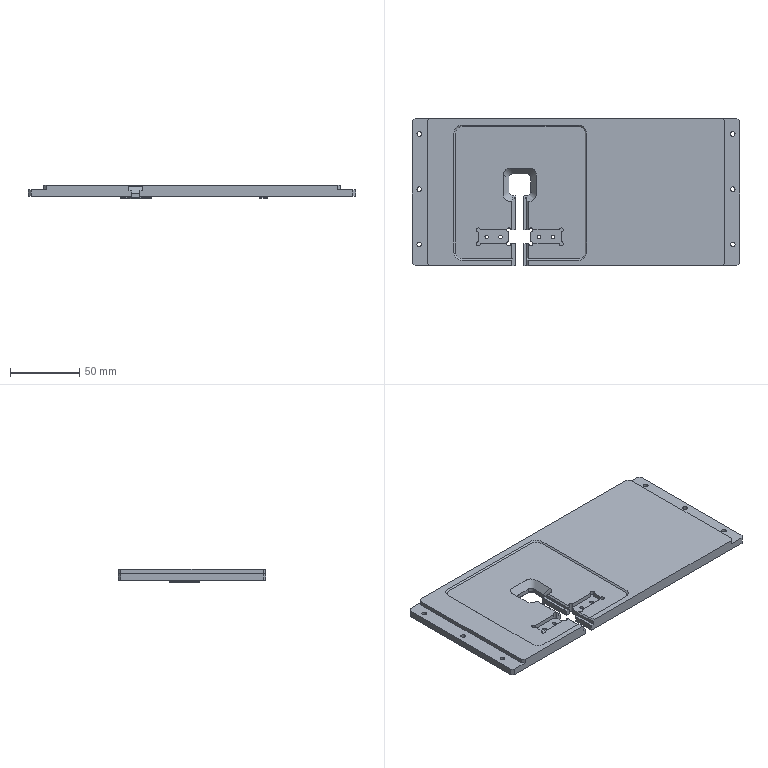NC program | NX | posted with a generic post | part box 237 x 107 x 9.5 mm
Lines 1381 to 3550 of 4908, first 1673 of 2168 lines:
(CAVITY_MILL_COPY_COPY_1 , TOOL : D6)
N2754 T06 M6
N2756 G54
N2758 G17 G0 G90 X-10.869 Y3.1 S3800 M3
N2760 G43 Z30. H6
N2762 Z-0.6
N2764 G94 G1 Z-1.6 F1000.
N2766 X-11.158 Y3.6
N2768 G3 X-12.024 Y4.1 R1.
N2770 G1 X-13.63 F1650.
N2772 G3 X-14.03 Y3.7 R0.4
N2774 G1 Y2.094
N2776 G3 X-13.53 Y1.228 R1.
N2778 G1 X-13.03 Y0.939
N2780 Z-0.6
N2782 G0 Z30.
N2784 X-10.769 Y3.
N2786 Z-0.7
N2788 G1 Z-1.7 F1000.
N2790 X-11.058 Y3.5
N2792 G3 X-11.924 Y4. R1.
N2794 G1 X-13.63 F1650.
N2796 G3 X-13.93 Y3.7 R0.3
N2798 G1 Y1.994
N2800 G3 X-13.43 Y1.128 R1.
N2802 G1 X-12.93 Y0.839
N2804 Z-0.7
N2806 G0 Z30.
N2808 X-10.669 Y2.9
N2810 Z-0.8
N2812 G1 Z-1.8 F1000.
N2814 X-10.958 Y3.4
N2816 G3 X-11.824 Y3.9 R1.
N2818 G1 X-13.63 F1650.
N2820 G3 X-13.83 Y3.7 R0.2
N2822 G1 Y1.894
N2824 G3 X-13.33 Y1.028 R1.
N2826 G1 X-12.83 Y0.739
N2828 Z-0.8
N2830 G0 Z30.
N2832 X-10.569 Y2.8
N2834 Z-0.9
N2836 G1 Z-1.9 F1000.
N2838 X-10.858 Y3.3
N2840 G3 X-11.724 Y3.8 R1.
N2842 G1 X-13.63 F1650.
N2844 X-13.695 Y3.813
N2846 X-13.743 Y3.765
N2848 X-13.73 Y3.7
N2850 Y1.794
N2852 G3 X-13.23 Y0.928 R1.
N2854 G1 X-12.73 Y0.639
N2856 Z-0.9
N2858 G0 Z30.
N2860 X-10.476 Y2.708
N2862 Z-1.
N2864 G1 Z-2. F1000.
N2866 X-10.765 Y3.208
N2868 G3 X-11.631 Y3.708 R1.
N2870 G1 X-13.63 F1650.
N2872 X-13.638 Y3.7
N2874 Y1.701
N2876 G3 X-13.138 Y0.835 R1.
N2878 G1 X-12.638 Y0.546
N2880 Z-1.
N2882 G0 Z30.
N2884 X-10.469 Y2.7
N2886 Z-1.1
N2888 G1 Z-2.1 F1000.
N2890 X-10.758 Y3.2
N2892 G3 X-11.624 Y3.7 R1.
N2894 G1 X-13.63 F1650.
N2896 Y1.694
N2898 G3 X-13.13 Y0.828 R1.
N2900 G1 X-12.63 Y0.539
N2902 Z-1.1
N2904 G0 Z30.
N2906 X-10.469 Y2.7
N2908 Z-1.2
N2910 G1 Z-2.2 F1000.
N2912 X-10.758 Y3.2
N2914 G3 X-11.624 Y3.7 R1.
N2916 G1 X-13.63 F1650.
N2918 Y1.694
N2920 G3 X-13.13 Y0.828 R1.
N2922 G1 X-12.63 Y0.539
N2924 Z-1.2
N2926 G0 Z30.
N2928 X-10.469 Y2.7
N2930 Z-1.3
N2932 G1 Z-2.3 F1000.
N2934 X-10.758 Y3.2
N2936 G3 X-11.624 Y3.7 R1.
N2938 G1 X-13.63 F1650.
N2940 Y1.694
N2942 G3 X-13.13 Y0.828 R1.
N2944 G1 X-12.63 Y0.539
N2946 Z-1.3
N2948 G0 Z30.
N2950 X-10.469 Y2.7
N2952 Z-1.4
N2954 G1 Z-2.4 F1000.
N2956 X-10.758 Y3.2
N2958 G3 X-11.624 Y3.7 R1.
N2960 G1 X-13.63 F1650.
N2962 Y1.694
N2964 G3 X-13.13 Y0.828 R1.
N2966 G1 X-12.63 Y0.539
N2968 Z-1.4
N2970 G0 Z30.
N2972 X-10.469 Y2.7
N2974 Z-1.5
N2976 G1 Z-2.5 F1000.
N2978 X-10.758 Y3.2
N2980 G3 X-11.624 Y3.7 R1.
N2982 G1 X-13.63 F1650.
N2984 Y1.694
N2986 G3 X-13.13 Y0.828 R1.
N2988 G1 X-12.63 Y0.539
N2990 Z-1.5
N2992 G0 X-10.469 Y2.7 Z-1.6
N2994 G1 Z-2.6 F1000.
N2996 X-10.758 Y3.2
N2998 G3 X-11.624 Y3.7 R1.
N3000 G1 X-13.63 F1650.
N3002 Y1.694
N3004 G3 X-13.13 Y0.828 R1.
N3006 G1 X-12.63 Y0.539
N3008 Z-1.6
N3010 G0 X-10.469 Y2.7 Z-1.7
N3012 G1 Z-2.7 F1000.
N3014 X-10.758 Y3.2
N3016 G3 X-11.624 Y3.7 R1.
N3018 G1 X-13.63 F1650.
N3020 Y1.694
N3022 G3 X-13.13 Y0.828 R1.
N3024 G1 X-12.63 Y0.539
N3026 Z-1.7
N3028 G0 X-10.469 Y2.7 Z-1.8
N3030 G1 Z-2.8 F1000.
N3032 X-10.758 Y3.2
N3034 G3 X-11.624 Y3.7 R1.
N3036 G1 X-13.63 F1650.
N3038 Y1.694
N3040 G3 X-13.13 Y0.828 R1.
N3042 G1 X-12.63 Y0.539
N3044 Z-1.8
N3046 G0 X-10.469 Y2.7 Z-1.9
N3048 G1 Z-2.9 F1000.
N3050 X-10.758 Y3.2
N3052 G3 X-11.624 Y3.7 R1.
N3054 G1 X-13.63 F1650.
N3056 Y1.694
N3058 G3 X-13.13 Y0.828 R1.
N3060 G1 X-12.63 Y0.539
N3062 Z-1.9
N3064 G0 X-10.469 Y2.7 Z-2.
N3066 G1 Z-3. F1000.
N3068 X-10.758 Y3.2
N3070 G3 X-11.624 Y3.7 R1.
N3072 G1 X-13.63 F1650.
N3074 Y1.694
N3076 G3 X-13.13 Y0.828 R1.
N3078 G1 X-12.63 Y0.539
N3080 Z-2.
N3082 G0 X-10.469 Y2.7 Z-2.1
N3084 G1 Z-3.1 F1000.
N3086 X-10.758 Y3.2
N3088 G3 X-11.624 Y3.7 R1.
N3090 G1 X-13.63 F1650.
N3092 Y1.694
N3094 G3 X-13.13 Y0.828 R1.
N3096 G1 X-12.63 Y0.539
N3098 Z-2.1
N3100 G0 X-10.469 Y2.7 Z-2.2
N3102 G1 Z-3.2 F1000.
N3104 X-10.758 Y3.2
N3106 G3 X-11.624 Y3.7 R1.
N3108 G1 X-13.63 F1650.
N3110 Y1.694
N3112 G3 X-13.13 Y0.828 R1.
N3114 G1 X-12.63 Y0.539
N3116 Z-2.2
N3118 G0 X-10.469 Y2.7 Z-2.3
N3120 G1 Z-3.3 F1000.
N3122 X-10.758 Y3.2
N3124 G3 X-11.624 Y3.7 R1.
N3126 G1 X-13.63 F1650.
N3128 Y1.694
N3130 G3 X-13.13 Y0.828 R1.
N3132 G1 X-12.63 Y0.539
N3134 Z-2.3
N3136 G0 X-10.469 Y2.7 Z-2.4
N3138 G1 Z-3.4 F1000.
N3140 X-10.758 Y3.2
N3142 G3 X-11.624 Y3.7 R1.
N3144 G1 X-13.63 F1650.
N3146 Y1.694
N3148 G3 X-13.13 Y0.828 R1.
N3150 G1 X-12.63 Y0.539
N3152 Z-2.4
N3154 G0 X-10.469 Y2.7 Z-2.5
N3156 G1 Z-3.5 F1000.
N3158 X-10.758 Y3.2
N3160 G3 X-11.624 Y3.7 R1.
N3162 G1 X-13.63 F1650.
N3164 Y1.694
N3166 G3 X-13.13 Y0.828 R1.
N3168 G1 X-12.63 Y0.539
N3170 Z-2.5
N3172 G0 X-10.469 Y2.7 Z-2.6
N3174 G1 Z-3.6 F1000.
N3176 X-10.758 Y3.2
N3178 G3 X-11.624 Y3.7 R1.
N3180 G1 X-13.63 F1650.
N3182 Y1.694
N3184 G3 X-13.13 Y0.828 R1.
N3186 G1 X-12.63 Y0.539
N3188 Z-2.6
N3190 G0 X-10.469 Y2.7 Z-2.7
N3192 G1 Z-3.7 F1000.
N3194 X-10.758 Y3.2
N3196 G3 X-11.624 Y3.7 R1.
N3198 G1 X-13.63 F1650.
N3200 Y1.694
N3202 G3 X-13.13 Y0.828 R1.
N3204 G1 X-12.63 Y0.539
N3206 Z-2.7
N3208 G0 X-10.469 Y2.7 Z-2.8
N3210 G1 Z-3.8 F1000.
N3212 X-10.758 Y3.2
N3214 G3 X-11.624 Y3.7 R1.
N3216 G1 X-13.63 F1650.
N3218 Y1.694
N3220 G3 X-13.13 Y0.828 R1.
N3222 G1 X-12.63 Y0.539
N3224 Z-2.8
N3226 G0 X-10.469 Y2.7 Z-2.9
N3228 G1 Z-3.9 F1000.
N3230 X-10.758 Y3.2
N3232 G3 X-11.624 Y3.7 R1.
N3234 G1 X-13.63 F1650.
N3236 Y1.694
N3238 G3 X-13.13 Y0.828 R1.
N3240 G1 X-12.63 Y0.539
N3242 Z-2.9
N3244 G0 X-10.469 Y2.7 Z-3.
N3246 G1 Z-4. F1000.
N3248 X-10.758 Y3.2
N3250 G3 X-11.624 Y3.7 R1.
N3252 G1 X-13.63 F1650.
N3254 Y1.694
N3256 G3 X-13.13 Y0.828 R1.
N3258 G1 X-12.63 Y0.539
N3260 Z-3.
N3262 G0 X-10.469 Y2.7 Z-3.1
N3264 G1 Z-4.1 F1000.
N3266 X-10.758 Y3.2
N3268 G3 X-11.624 Y3.7 R1.
N3270 G1 X-13.63 F1650.
N3272 Y1.694
N3274 G3 X-13.13 Y0.828 R1.
N3276 G1 X-12.63 Y0.539
N3278 Z-3.1
N3280 G0 X-10.469 Y2.7 Z-3.2
N3282 G1 Z-4.2 F1000.
N3284 X-10.758 Y3.2
N3286 G3 X-11.624 Y3.7 R1.
N3288 G1 X-13.63 F1650.
N3290 Y1.694
N3292 G3 X-13.13 Y0.828 R1.
N3294 G1 X-12.63 Y0.539
N3296 Z-3.2
N3298 G0 X-10.469 Y2.7 Z-3.3
N3300 G1 Z-4.3 F1000.
N3302 X-10.758 Y3.2
N3304 G3 X-11.624 Y3.7 R1.
N3306 G1 X-13.63 F1650.
N3308 Y1.694
N3310 G3 X-13.13 Y0.828 R1.
N3312 G1 X-12.63 Y0.539
N3314 Z-3.3
N3316 G0 X-10.469 Y2.7 Z-3.4
N3318 G1 Z-4.4 F1000.
N3320 X-10.758 Y3.2
N3322 G3 X-11.624 Y3.7 R1.
N3324 G1 X-13.63 F1650.
N3326 Y1.694
N3328 G3 X-13.13 Y0.828 R1.
N3330 G1 X-12.63 Y0.539
N3332 Z-3.4
N3334 G0 X-10.469 Y2.7 Z-3.5
N3336 G1 Z-4.5 F1000.
N3338 X-10.758 Y3.2
N3340 G3 X-11.624 Y3.7 R1.
N3342 G1 X-13.63 F1650.
N3344 Y1.694
N3346 G3 X-13.13 Y0.828 R1.
N3348 G1 X-12.63 Y0.539
N3350 Z-3.5
N3352 G0 X-10.469 Y2.7 Z-3.6
N3354 G1 Z-4.6 F1000.
N3356 X-10.758 Y3.2
N3358 G3 X-11.624 Y3.7 R1.
N3360 G1 X-13.63 F1650.
N3362 Y1.694
N3364 G3 X-13.13 Y0.828 R1.
N3366 G1 X-12.63 Y0.539
N3368 Z-3.6
N3370 G0 X-10.469 Y2.7 Z-3.7
N3372 G1 Z-4.7 F1000.
N3374 X-10.758 Y3.2
N3376 G3 X-11.624 Y3.7 R1.
N3378 G1 X-13.63 F1650.
N3380 Y1.694
N3382 G3 X-13.13 Y0.828 R1.
N3384 G1 X-12.63 Y0.539
N3386 Z-3.7
N3388 G0 X-10.469 Y2.7 Z-3.8
N3390 G1 Z-4.8 F1000.
N3392 X-10.758 Y3.2
N3394 G3 X-11.624 Y3.7 R1.
N3396 G1 X-13.63 F1650.
N3398 Y1.694
N3400 G3 X-13.13 Y0.828 R1.
N3402 G1 X-12.63 Y0.539
N3404 Z-3.8
N3406 G0 X-10.469 Y2.7 Z-3.9
N3408 G1 Z-4.9 F1000.
N3410 X-10.758 Y3.2
N3412 G3 X-11.624 Y3.7 R1.
N3414 G1 X-13.63 F1650.
N3416 Y1.694
N3418 G3 X-13.13 Y0.828 R1.
N3420 G1 X-12.63 Y0.539
N3422 Z-3.9
N3424 G0 X-10.469 Y2.7 Z-4.
N3426 G1 Z-5. F1000.
N3428 X-10.758 Y3.2
N3430 G3 X-11.624 Y3.7 R1.
N3432 G1 X-13.63 F1650.
N3434 Y1.694
N3436 G3 X-13.13 Y0.828 R1.
N3438 G1 X-12.63 Y0.539
N3440 Z-4.
N3442 G0 X-10.469 Y2.7 Z-4.1
N3444 G1 Z-5.1 F1000.
N3446 X-10.758 Y3.2
N3448 G3 X-11.624 Y3.7 R1.
N3450 G1 X-13.63 F1650.
N3452 Y1.694
N3454 G3 X-13.13 Y0.828 R1.
N3456 G1 X-12.63 Y0.539
N3458 Z-4.1
N3460 G0 X-10.469 Y2.7 Z-4.2
N3462 G1 Z-5.2 F1000.
N3464 X-10.758 Y3.2
N3466 G3 X-11.624 Y3.7 R1.
N3468 G1 X-13.63 F1650.
N3470 Y1.694
N3472 G3 X-13.13 Y0.828 R1.
N3474 G1 X-12.63 Y0.539
N3476 Z-4.2
N3478 G0 X-10.469 Y2.7 Z-4.3
N3480 G1 Z-5.3 F1000.
N3482 X-10.758 Y3.2
N3484 G3 X-11.624 Y3.7 R1.
N3486 G1 X-13.63 F1650.
N3488 Y1.694
N3490 G3 X-13.13 Y0.828 R1.
N3492 G1 X-12.63 Y0.539
N3494 Z-4.3
N3496 G0 X-10.469 Y2.7 Z-4.4
N3498 G1 Z-5.4 F1000.
N3500 X-10.758 Y3.2
N3502 G3 X-11.624 Y3.7 R1.
N3504 G1 X-13.63 F1650.
N3506 Y1.694
N3508 G3 X-13.13 Y0.828 R1.
N3510 G1 X-12.63 Y0.539
N3512 Z-4.4
N3514 G0 X-10.469 Y2.7 Z-4.5
N3516 G1 Z-5.5 F1000.
N3518 X-10.758 Y3.2
N3520 G3 X-11.624 Y3.7 R1.
N3522 G1 X-13.63 F1650.
N3524 Y1.694
N3526 G3 X-13.13 Y0.828 R1.
N3528 G1 X-12.63 Y0.539
N3530 Z-4.5
N3532 G0 X-10.469 Y2.7 Z-4.6
N3534 G1 Z-5.6 F1000.
N3536 X-10.758 Y3.2
N3538 G3 X-11.624 Y3.7 R1.
N3540 G1 X-13.63 F1650.
N3542 Y1.694
N3544 G3 X-13.13 Y0.828 R1.
N3546 G1 X-12.63 Y0.539
N3548 Z-4.6
N3550 G0 X-10.469 Y2.7 Z-4.7
N3552 G1 Z-5.7 F1000.
N3554 X-10.758 Y3.2
N3556 G3 X-11.624 Y3.7 R1.
N3558 G1 X-13.63 F1650.
N3560 Y1.694
N3562 G3 X-13.13 Y0.828 R1.
N3564 G1 X-12.63 Y0.539
N3566 Z-4.7
N3568 G0 X-10.469 Y2.7 Z-4.8
N3570 G1 Z-5.8 F1000.
N3572 X-10.758 Y3.2
N3574 G3 X-11.624 Y3.7 R1.
N3576 G1 X-13.63 F1650.
N3578 Y1.694
N3580 G3 X-13.13 Y0.828 R1.
N3582 G1 X-12.63 Y0.539
N3584 Z-4.8
N3586 G0 X-10.469 Y2.7 Z-4.9
N3588 G1 Z-5.9 F1000.
N3590 X-10.758 Y3.2
N3592 G3 X-11.624 Y3.7 R1.
N3594 G1 X-13.63 F1650.
N3596 Y1.694
N3598 G3 X-13.13 Y0.828 R1.
N3600 G1 X-12.63 Y0.539
N3602 Z-4.9
N3604 G0 X-10.469 Y2.7 Z-5.
N3606 G1 Z-6. F1000.
N3608 X-10.758 Y3.2
N3610 G3 X-11.624 Y3.7 R1.
N3612 G1 X-13.63 F1650.
N3614 Y1.694
N3616 G3 X-13.13 Y0.828 R1.
N3618 G1 X-12.63 Y0.539
N3620 Z-5.
N3622 G0 X-10.469 Y2.7 Z-5.1
N3624 G1 Z-6.1 F1000.
N3626 X-10.758 Y3.2
N3628 G3 X-11.624 Y3.7 R1.
N3630 G1 X-13.63 F1650.
N3632 Y1.694
N3634 G3 X-13.13 Y0.828 R1.
N3636 G1 X-12.63 Y0.539
N3638 Z-5.1
N3640 G0 X-10.469 Y2.7 Z-5.2
N3642 G1 Z-6.2 F1000.
N3644 X-10.758 Y3.2
N3646 G3 X-11.624 Y3.7 R1.
N3648 G1 X-13.63 F1650.
N3650 Y1.694
N3652 G3 X-13.13 Y0.828 R1.
N3654 G1 X-12.63 Y0.539
N3656 Z-5.2
N3658 G0 X-10.469 Y2.7 Z-5.3
N3660 G1 Z-6.3 F1000.
N3662 X-10.758 Y3.2
N3664 G3 X-11.624 Y3.7 R1.
N3666 G1 X-13.63 F1650.
N3668 Y1.694
N3670 G3 X-13.13 Y0.828 R1.
N3672 G1 X-12.63 Y0.539
N3674 Z-5.3
N3676 G0 X-10.469 Y2.7 Z-5.4
N3678 G1 Z-6.4 F1000.
N3680 X-10.758 Y3.2
N3682 G3 X-11.624 Y3.7 R1.
N3684 G1 X-13.63 F1650.
N3686 Y1.694
N3688 G3 X-13.13 Y0.828 R1.
N3690 G1 X-12.63 Y0.539
N3692 Z-5.4
N3694 G0 X-10.469 Y2.7 Z-5.5
N3696 G1 Z-6.5 F1000.
N3698 X-10.758 Y3.2
N3700 G3 X-11.624 Y3.7 R1.
N3702 G1 X-13.63 F1650.
N3704 Y1.694
N3706 G3 X-13.13 Y0.828 R1.
N3708 G1 X-12.63 Y0.539
N3710 Z-5.5
N3712 G0 X-10.469 Y2.7 Z-5.6
N3714 G1 Z-6.6 F1000.
N3716 X-10.758 Y3.2
N3718 G3 X-11.624 Y3.7 R1.
N3720 G1 X-13.63 F1650.
N3722 Y1.694
N3724 G3 X-13.13 Y0.828 R1.
N3726 G1 X-12.63 Y0.539
N3728 Z-5.6
N3730 G0 X-10.469 Y2.7 Z-5.7
N3732 G1 Z-6.7 F1000.
N3734 X-10.758 Y3.2
N3736 G3 X-11.624 Y3.7 R1.
N3738 G1 X-13.63 F1650.
N3740 Y1.694
N3742 G3 X-13.13 Y0.828 R1.
N3744 G1 X-12.63 Y0.539
N3746 Z-5.7
N3748 G0 X-10.469 Y2.7 Z-5.8
N3750 G1 Z-6.8 F1000.
N3752 X-10.758 Y3.2
N3754 G3 X-11.624 Y3.7 R1.
N3756 G1 X-13.63 F1650.
N3758 Y1.694
N3760 G3 X-13.13 Y0.828 R1.
N3762 G1 X-12.63 Y0.539
N3764 Z-5.8
N3766 G0 X-10.469 Y2.7 Z-5.9
N3768 G1 Z-6.9 F1000.
N3770 X-10.758 Y3.2
N3772 G3 X-11.624 Y3.7 R1.
N3774 G1 X-13.63 F1650.
N3776 Y1.694
N3778 G3 X-13.13 Y0.828 R1.
N3780 G1 X-12.63 Y0.539
N3782 Z-5.9
N3784 G0 X-10.469 Y2.7 Z-6.
N3786 G1 Z-7. F1000.
N3788 X-10.758 Y3.2
N3790 G3 X-11.624 Y3.7 R1.
N3792 G1 X-13.63 F1650.
N3794 Y1.694
N3796 G3 X-13.13 Y0.828 R1.
N3798 G1 X-12.63 Y0.539
N3800 Z-6.
N3802 G0 Z30.
N3804 X-13.03 Y-11.539
N3806 Z-0.6
N3808 G1 Z-1.6 F1000.
N3810 X-13.53 Y-11.828
N3812 G3 X-14.03 Y-12.694 R1.
N3814 G1 Y-14.3 F1650.
N3816 G3 X-13.63 Y-14.7 R0.4
N3818 G1 X-12.024
N3820 G3 X-11.158 Y-14.2 R1.
N3822 G1 X-10.869 Y-13.7
N3824 Z-0.6
N3826 G0 Z30.
N3828 X-12.93 Y-11.439
N3830 Z-0.7
N3832 G1 Z-1.7 F1000.
N3834 X-13.43 Y-11.728
N3836 G3 X-13.93 Y-12.594 R1.
N3838 G1 Y-14.3 F1650.
N3840 G3 X-13.63 Y-14.6 R0.3
N3842 G1 X-11.924
N3844 G3 X-11.058 Y-14.1 R1.
N3846 G1 X-10.769 Y-13.6
N3848 Z-0.7
N3850 G0 Z30.
N3852 X-12.83 Y-11.339
N3854 Z-0.8
N3856 G1 Z-1.8 F1000.
N3858 X-13.33 Y-11.628
N3860 G3 X-13.83 Y-12.494 R1.
N3862 G1 Y-14.3 F1650.
N3864 G3 X-13.63 Y-14.5 R0.2
N3866 G1 X-11.824
N3868 G3 X-10.958 Y-14. R1.
N3870 G1 X-10.669 Y-13.5
N3872 Z-0.8
N3874 G0 Z30.
N3876 X-12.73 Y-11.239
N3878 Z-0.9
N3880 G1 Z-1.9 F1000.
N3882 X-13.23 Y-11.528
N3884 G3 X-13.73 Y-12.394 R1.
N3886 G1 Y-14.3 F1650.
N3888 X-13.743 Y-14.365
N3890 X-13.695 Y-14.413
N3892 X-13.63 Y-14.4
N3894 X-11.724
N3896 G3 X-10.858 Y-13.9 R1.
N3898 G1 X-10.569 Y-13.4
N3900 Z-0.9
N3902 G0 Z30.
N3904 X-12.638 Y-11.146
N3906 Z-1.
N3908 G1 Z-2. F1000.
N3910 X-13.138 Y-11.435
N3912 G3 X-13.638 Y-12.301 R1.
N3914 G1 Y-14.3 F1650.
N3916 X-13.63 Y-14.308
N3918 X-11.631
N3920 G3 X-10.765 Y-13.808 R1.
N3922 G1 X-10.476 Y-13.308
N3924 Z-1.
N3926 G0 Z30.
N3928 X-12.63 Y-11.139
N3930 Z-1.1
N3932 G1 Z-2.1 F1000.
N3934 X-13.13 Y-11.428
N3936 G3 X-13.63 Y-12.294 R1.
N3938 G1 Y-14.3 F1650.
N3940 X-11.624
N3942 G3 X-10.758 Y-13.8 R1.
N3944 G1 X-10.469 Y-13.3
N3946 Z-1.1
N3948 G0 Z30.
N3950 X-12.63 Y-11.139
N3952 Z-1.2
N3954 G1 Z-2.2 F1000.
N3956 X-13.13 Y-11.428
N3958 G3 X-13.63 Y-12.294 R1.
N3960 G1 Y-14.3 F1650.
N3962 X-11.624
N3964 G3 X-10.758 Y-13.8 R1.
N3966 G1 X-10.469 Y-13.3
N3968 Z-1.2
N3970 G0 Z30.
N3972 X-12.63 Y-11.139
N3974 Z-1.3
N3976 G1 Z-2.3 F1000.
N3978 X-13.13 Y-11.428
N3980 G3 X-13.63 Y-12.294 R1.
N3982 G1 Y-14.3 F1650.
N3984 X-11.624
N3986 G3 X-10.758 Y-13.8 R1.
N3988 G1 X-10.469 Y-13.3
N3990 Z-1.3
N3992 G0 Z30.
N3994 X-12.63 Y-11.139
N3996 Z-1.4
N3998 G1 Z-2.4 F1000.
N4000 X-13.13 Y-11.428
N4002 G3 X-13.63 Y-12.294 R1.
N4004 G1 Y-14.3 F1650.
N4006 X-11.624
N4008 G3 X-10.758 Y-13.8 R1.
N4010 G1 X-10.469 Y-13.3
N4012 Z-1.4
N4014 G0 Z30.
N4016 X-12.63 Y-11.139
N4018 Z-1.5
N4020 G1 Z-2.5 F1000.
N4022 X-13.13 Y-11.428
N4024 G3 X-13.63 Y-12.294 R1.
N4026 G1 Y-14.3 F1650.
N4028 X-11.624
N4030 G3 X-10.758 Y-13.8 R1.
N4032 G1 X-10.469 Y-13.3
N4034 Z-1.5
N4036 G0 X-12.63 Y-11.139 Z-1.6
N4038 G1 Z-2.6 F1000.
N4040 X-13.13 Y-11.428
N4042 G3 X-13.63 Y-12.294 R1.
N4044 G1 Y-14.3 F1650.
N4046 X-11.624
N4048 G3 X-10.758 Y-13.8 R1.
N4050 G1 X-10.469 Y-13.3
N4052 Z-1.6
N4054 G0 X-12.63 Y-11.139 Z-1.7
N4056 G1 Z-2.7 F1000.
N4058 X-13.13 Y-11.428
N4060 G3 X-13.63 Y-12.294 R1.
N4062 G1 Y-14.3 F1650.
N4064 X-11.624
N4066 G3 X-10.758 Y-13.8 R1.
N4068 G1 X-10.469 Y-13.3
N4070 Z-1.7
N4072 G0 X-12.63 Y-11.139 Z-1.8
N4074 G1 Z-2.8 F1000.
N4076 X-13.13 Y-11.428
N4078 G3 X-13.63 Y-12.294 R1.
N4080 G1 Y-14.3 F1650.
N4082 X-11.624
N4084 G3 X-10.758 Y-13.8 R1.
N4086 G1 X-10.469 Y-13.3
N4088 Z-1.8
N4090 G0 X-12.63 Y-11.139 Z-1.9
N4092 G1 Z-2.9 F1000.
N4094 X-13.13 Y-11.428
N4096 G3 X-13.63 Y-12.294 R1.
N4098 G1 Y-14.3 F1650.
N4100 X-11.624
N4102 G3 X-10.758 Y-13.8 R1.
N4104 G1 X-10.469 Y-13.3
N4106 Z-1.9
N4108 G0 X-12.63 Y-11.139 Z-2.
N4110 G1 Z-3. F1000.
N4112 X-13.13 Y-11.428
N4114 G3 X-13.63 Y-12.294 R1.
N4116 G1 Y-14.3 F1650.
N4118 X-11.624
N4120 G3 X-10.758 Y-13.8 R1.
N4122 G1 X-10.469 Y-13.3
N4124 Z-2.
N4126 G0 X-12.63 Y-11.139 Z-2.1
N4128 G1 Z-3.1 F1000.
N4130 X-13.13 Y-11.428
N4132 G3 X-13.63 Y-12.294 R1.
N4134 G1 Y-14.3 F1650.
N4136 X-11.624
N4138 G3 X-10.758 Y-13.8 R1.
N4140 G1 X-10.469 Y-13.3
N4142 Z-2.1
N4144 G0 X-12.63 Y-11.139 Z-2.2
N4146 G1 Z-3.2 F1000.
N4148 X-13.13 Y-11.428
N4150 G3 X-13.63 Y-12.294 R1.
N4152 G1 Y-14.3 F1650.
N4154 X-11.624
N4156 G3 X-10.758 Y-13.8 R1.
N4158 G1 X-10.469 Y-13.3
N4160 Z-2.2
N4162 G0 X-12.63 Y-11.139 Z-2.3
N4164 G1 Z-3.3 F1000.
N4166 X-13.13 Y-11.428
N4168 G3 X-13.63 Y-12.294 R1.
N4170 G1 Y-14.3 F1650.
N4172 X-11.624
N4174 G3 X-10.758 Y-13.8 R1.
N4176 G1 X-10.469 Y-13.3
N4178 Z-2.3
N4180 G0 X-12.63 Y-11.139 Z-2.4
N4182 G1 Z-3.4 F1000.
N4184 X-13.13 Y-11.428
N4186 G3 X-13.63 Y-12.294 R1.
N4188 G1 Y-14.3 F1650.
N4190 X-11.624
N4192 G3 X-10.758 Y-13.8 R1.
N4194 G1 X-10.469 Y-13.3
N4196 Z-2.4
N4198 G0 X-12.63 Y-11.139 Z-2.5
N4200 G1 Z-3.5 F1000.
N4202 X-13.13 Y-11.428
N4204 G3 X-13.63 Y-12.294 R1.
N4206 G1 Y-14.3 F1650.
N4208 X-11.624
N4210 G3 X-10.758 Y-13.8 R1.
N4212 G1 X-10.469 Y-13.3
N4214 Z-2.5
N4216 G0 X-12.63 Y-11.139 Z-2.6
N4218 G1 Z-3.6 F1000.
N4220 X-13.13 Y-11.428
N4222 G3 X-13.63 Y-12.294 R1.
N4224 G1 Y-14.3 F1650.
N4226 X-11.624
N4228 G3 X-10.758 Y-13.8 R1.
N4230 G1 X-10.469 Y-13.3
N4232 Z-2.6
N4234 G0 X-12.63 Y-11.139 Z-2.7
N4236 G1 Z-3.7 F1000.
N4238 X-13.13 Y-11.428
N4240 G3 X-13.63 Y-12.294 R1.
N4242 G1 Y-14.3 F1650.
N4244 X-11.624
N4246 G3 X-10.758 Y-13.8 R1.
N4248 G1 X-10.469 Y-13.3
N4250 Z-2.7
N4252 G0 X-12.63 Y-11.139 Z-2.8
N4254 G1 Z-3.8 F1000.
N4256 X-13.13 Y-11.428
N4258 G3 X-13.63 Y-12.294 R1.
N4260 G1 Y-14.3 F1650.
N4262 X-11.624
N4264 G3 X-10.758 Y-13.8 R1.
N4266 G1 X-10.469 Y-13.3
N4268 Z-2.8
N4270 G0 X-12.63 Y-11.139 Z-2.9
N4272 G1 Z-3.9 F1000.
N4274 X-13.13 Y-11.428
N4276 G3 X-13.63 Y-12.294 R1.
N4278 G1 Y-14.3 F1650.
N4280 X-11.624
N4282 G3 X-10.758 Y-13.8 R1.
N4284 G1 X-10.469 Y-13.3
N4286 Z-2.9
N4288 G0 X-12.63 Y-11.139 Z-3.
N4290 G1 Z-4. F1000.
N4292 X-13.13 Y-11.428
N4294 G3 X-13.63 Y-12.294 R1.
N4296 G1 Y-14.3 F1650.
N4298 X-11.624
N4300 G3 X-10.758 Y-13.8 R1.
N4302 G1 X-10.469 Y-13.3
N4304 Z-3.
N4306 G0 X-12.63 Y-11.139 Z-3.1
N4308 G1 Z-4.1 F1000.
N4310 X-13.13 Y-11.428
N4312 G3 X-13.63 Y-12.294 R1.
N4314 G1 Y-14.3 F1650.
N4316 X-11.624
N4318 G3 X-10.758 Y-13.8 R1.
N4320 G1 X-10.469 Y-13.3
N4322 Z-3.1
N4324 G0 X-12.63 Y-11.139 Z-3.2
N4326 G1 Z-4.2 F1000.
N4328 X-13.13 Y-11.428
N4330 G3 X-13.63 Y-12.294 R1.
N4332 G1 Y-14.3 F1650.
N4334 X-11.624
N4336 G3 X-10.758 Y-13.8 R1.
N4338 G1 X-10.469 Y-13.3
N4340 Z-3.2
N4342 G0 X-12.63 Y-11.139 Z-3.3
N4344 G1 Z-4.3 F1000.
N4346 X-13.13 Y-11.428
N4348 G3 X-13.63 Y-12.294 R1.
N4350 G1 Y-14.3 F1650.
N4352 X-11.624
N4354 G3 X-10.758 Y-13.8 R1.
N4356 G1 X-10.469 Y-13.3
N4358 Z-3.3
N4360 G0 X-12.63 Y-11.139 Z-3.4
N4362 G1 Z-4.4 F1000.
N4364 X-13.13 Y-11.428
N4366 G3 X-13.63 Y-12.294 R1.
N4368 G1 Y-14.3 F1650.
N4370 X-11.624
N4372 G3 X-10.758 Y-13.8 R1.
N4374 G1 X-10.469 Y-13.3
N4376 Z-3.4
N4378 G0 X-12.63 Y-11.139 Z-3.5
N4380 G1 Z-4.5 F1000.
N4382 X-13.13 Y-11.428
N4384 G3 X-13.63 Y-12.294 R1.
N4386 G1 Y-14.3 F1650.
N4388 X-11.624
N4390 G3 X-10.758 Y-13.8 R1.
N4392 G1 X-10.469 Y-13.3
N4394 Z-3.5
N4396 G0 X-12.63 Y-11.139 Z-3.6
N4398 G1 Z-4.6 F1000.
N4400 X-13.13 Y-11.428
N4402 G3 X-13.63 Y-12.294 R1.
N4404 G1 Y-14.3 F1650.
N4406 X-11.624
N4408 G3 X-10.758 Y-13.8 R1.
N4410 G1 X-10.469 Y-13.3
N4412 Z-3.6
N4414 G0 X-12.63 Y-11.139 Z-3.7
N4416 G1 Z-4.7 F1000.
N4418 X-13.13 Y-11.428
N4420 G3 X-13.63 Y-12.294 R1.
N4422 G1 Y-14.3 F1650.
N4424 X-11.624
N4426 G3 X-10.758 Y-13.8 R1.
N4428 G1 X-10.469 Y-13.3
N4430 Z-3.7
N4432 G0 X-12.63 Y-11.139 Z-3.8
N4434 G1 Z-4.8 F1000.
N4436 X-13.13 Y-11.428
N4438 G3 X-13.63 Y-12.294 R1.
N4440 G1 Y-14.3 F1650.
N4442 X-11.624
N4444 G3 X-10.758 Y-13.8 R1.
N4446 G1 X-10.469 Y-13.3
N4448 Z-3.8
N4450 G0 X-12.63 Y-11.139 Z-3.9
N4452 G1 Z-4.9 F1000.
N4454 X-13.13 Y-11.428
N4456 G3 X-13.63 Y-12.294 R1.
N4458 G1 Y-14.3 F1650.
N4460 X-11.624
N4462 G3 X-10.758 Y-13.8 R1.
N4464 G1 X-10.469 Y-13.3
N4466 Z-3.9
N4468 G0 X-12.63 Y-11.139 Z-4.
N4470 G1 Z-5. F1000.
N4472 X-13.13 Y-11.428
N4474 G3 X-13.63 Y-12.294 R1.
N4476 G1 Y-14.3 F1650.
N4478 X-11.624
N4480 G3 X-10.758 Y-13.8 R1.
N4482 G1 X-10.469 Y-13.3
N4484 Z-4.
N4486 G0 X-12.63 Y-11.139 Z-4.1
N4488 G1 Z-5.1 F1000.
N4490 X-13.13 Y-11.428
N4492 G3 X-13.63 Y-12.294 R1.
N4494 G1 Y-14.3 F1650.
N4496 X-11.624
N4498 G3 X-10.758 Y-13.8 R1.
N4500 G1 X-10.469 Y-13.3
N4502 Z-4.1
N4504 G0 X-12.63 Y-11.139 Z-4.2
N4506 G1 Z-5.2 F1000.
N4508 X-13.13 Y-11.428
N4510 G3 X-13.63 Y-12.294 R1.
N4512 G1 Y-14.3 F1650.
N4514 X-11.624
N4516 G3 X-10.758 Y-13.8 R1.
N4518 G1 X-10.469 Y-13.3
N4520 Z-4.2
N4522 G0 X-12.63 Y-11.139 Z-4.3
N4524 G1 Z-5.3 F1000.
N4526 X-13.13 Y-11.428
N4528 G3 X-13.63 Y-12.294 R1.
N4530 G1 Y-14.3 F1650.
N4532 X-11.624
N4534 G3 X-10.758 Y-13.8 R1.
N4536 G1 X-10.469 Y-13.3
N4538 Z-4.3
N4540 G0 X-12.63 Y-11.139 Z-4.4
N4542 G1 Z-5.4 F1000.
N4544 X-13.13 Y-11.428
N4546 G3 X-13.63 Y-12.294 R1.
N4548 G1 Y-14.3 F1650.
N4550 X-11.624
N4552 G3 X-10.758 Y-13.8 R1.
N4554 G1 X-10.469 Y-13.3
N4556 Z-4.4
N4558 G0 X-12.63 Y-11.139 Z-4.5
N4560 G1 Z-5.5 F1000.
N4562 X-13.13 Y-11.428
N4564 G3 X-13.63 Y-12.294 R1.
N4566 G1 Y-14.3 F1650.
N4568 X-11.624
N4570 G3 X-10.758 Y-13.8 R1.
N4572 G1 X-10.469 Y-13.3
N4574 Z-4.5
N4576 G0 X-12.63 Y-11.139 Z-4.6
N4578 G1 Z-5.6 F1000.
N4580 X-13.13 Y-11.428
N4582 G3 X-13.63 Y-12.294 R1.
N4584 G1 Y-14.3 F1650.
N4586 X-11.624
N4588 G3 X-10.758 Y-13.8 R1.
N4590 G1 X-10.469 Y-13.3
N4592 Z-4.6
N4594 G0 X-12.63 Y-11.139 Z-4.7
N4596 G1 Z-5.7 F1000.
N4598 X-13.13 Y-11.428
N4600 G3 X-13.63 Y-12.294 R1.
N4602 G1 Y-14.3 F1650.
N4604 X-11.624
N4606 G3 X-10.758 Y-13.8 R1.
N4608 G1 X-10.469 Y-13.3
N4610 Z-4.7
N4612 G0 X-12.63 Y-11.139 Z-4.8
N4614 G1 Z-5.8 F1000.
N4616 X-13.13 Y-11.428
N4618 G3 X-13.63 Y-12.294 R1.
N4620 G1 Y-14.3 F1650.
N4622 X-11.624
N4624 G3 X-10.758 Y-13.8 R1.
N4626 G1 X-10.469 Y-13.3
N4628 Z-4.8
N4630 G0 X-12.63 Y-11.139 Z-4.9
N4632 G1 Z-5.9 F1000.
N4634 X-13.13 Y-11.428
N4636 G3 X-13.63 Y-12.294 R1.
N4638 G1 Y-14.3 F1650.
N4640 X-11.624
N4642 G3 X-10.758 Y-13.8 R1.
N4644 G1 X-10.469 Y-13.3
N4646 Z-4.9
N4648 G0 X-12.63 Y-11.139 Z-5.
N4650 G1 Z-6. F1000.
N4652 X-13.13 Y-11.428
N4654 G3 X-13.63 Y-12.294 R1.
N4656 G1 Y-14.3 F1650.
N4658 X-11.624
N4660 G3 X-10.758 Y-13.8 R1.
N4662 G1 X-10.469 Y-13.3
N4664 Z-5.
N4666 G0 X-12.63 Y-11.139 Z-5.1
N4668 G1 Z-6.1 F1000.
N4670 X-13.13 Y-11.428
N4672 G3 X-13.63 Y-12.294 R1.
N4674 G1 Y-14.3 F1650.
N4676 X-11.624
N4678 G3 X-10.758 Y-13.8 R1.
N4680 G1 X-10.469 Y-13.3
N4682 Z-5.1
N4684 G0 X-12.63 Y-11.139 Z-5.2
N4686 G1 Z-6.2 F1000.
N4688 X-13.13 Y-11.428
N4690 G3 X-13.63 Y-12.294 R1.
N4692 G1 Y-14.3 F1650.
N4694 X-11.624
N4696 G3 X-10.758 Y-13.8 R1.
N4698 G1 X-10.469 Y-13.3
N4700 Z-5.2
N4702 G0 X-12.63 Y-11.139 Z-5.3
N4704 G1 Z-6.3 F1000.
N4706 X-13.13 Y-11.428
N4708 G3 X-13.63 Y-12.294 R1.
N4710 G1 Y-14.3 F1650.
N4712 X-11.624
N4714 G3 X-10.758 Y-13.8 R1.
N4716 G1 X-10.469 Y-13.3
N4718 Z-5.3
N4720 G0 X-12.63 Y-11.139 Z-5.4
N4722 G1 Z-6.4 F1000.
N4724 X-13.13 Y-11.428
N4726 G3 X-13.63 Y-12.294 R1.
N4728 G1 Y-14.3 F1650.
N4730 X-11.624
N4732 G3 X-10.758 Y-13.8 R1.
N4734 G1 X-10.469 Y-13.3
N4736 Z-5.4
N4738 G0 X-12.63 Y-11.139 Z-5.5
N4740 G1 Z-6.5 F1000.
N4742 X-13.13 Y-11.428
N4744 G3 X-13.63 Y-12.294 R1.
N4746 G1 Y-14.3 F1650.
N4748 X-11.624
N4750 G3 X-10.758 Y-13.8 R1.
N4752 G1 X-10.469 Y-13.3
N4754 Z-5.5
N4756 G0 X-12.63 Y-11.139 Z-5.6
N4758 G1 Z-6.6 F1000.
N4760 X-13.13 Y-11.428
N4762 G3 X-13.63 Y-12.294 R1.
N4764 G1 Y-14.3 F1650.
N4766 X-11.624
N4768 G3 X-10.758 Y-13.8 R1.
N4770 G1 X-10.469 Y-13.3
N4772 Z-5.6
N4774 G0 X-12.63 Y-11.139 Z-5.7
N4776 G1 Z-6.7 F1000.
N4778 X-13.13 Y-11.428
N4780 G3 X-13.63 Y-12.294 R1.
N4782 G1 Y-14.3 F1650.
N4784 X-11.624
N4786 G3 X-10.758 Y-13.8 R1.
N4788 G1 X-10.469 Y-13.3
N4790 Z-5.7
N4792 G0 X-12.63 Y-11.139 Z-5.8
N4794 G1 Z-6.8 F1000.
N4796 X-13.13 Y-11.428
N4798 G3 X-13.63 Y-12.294 R1.
N4800 G1 Y-14.3 F1650.
N4802 X-11.624
N4804 G3 X-10.758 Y-13.8 R1.
N4806 G1 X-10.469 Y-13.3
N4808 Z-5.8
N4810 G0 X-12.63 Y-11.139 Z-5.9
N4812 G1 Z-6.9 F1000.
N4814 X-13.13 Y-11.428
N4816 G3 X-13.63 Y-12.294 R1.
N4818 G1 Y-14.3 F1650.
N4820 X-11.624
N4822 G3 X-10.758 Y-13.8 R1.
N4824 G1 X-10.469 Y-13.3
N4826 Z-5.9
N4828 G0 X-12.63 Y-11.139 Z-6.
N4830 G1 Z-7. F1000.
N4832 X-13.13 Y-11.428
N4834 G3 X-13.63 Y-12.294 R1.
N4836 G1 Y-14.3 F1650.
N4838 X-11.624
N4840 G3 X-10.758 Y-13.8 R1.
N4842 G1 X-10.469 Y-13.3
N4844 Z-6.
N4846 G0 Z30.
N4848 X40.609 Y-13.7
N4850 Z-0.6
N4852 G1 Z-1.6 F1000.
N4854 X40.898 Y-14.2
N4856 G3 X41.764 Y-14.7 R1.
N4858 G1 X43.37 F1650.
N4860 G3 X43.77 Y-14.3 R0.4
N4862 G1 Y-12.694
N4864 G3 X43.27 Y-11.828 R1.
N4866 G1 X42.77 Y-11.539
N4868 Z-0.6
N4870 G0 Z30.
N4872 X40.509 Y-13.6
N4874 Z-0.7
N4876 G1 Z-1.7 F1000.
N4878 X40.798 Y-14.1
N4880 G3 X41.664 Y-14.6 R1.
N4882 G1 X43.37 F1650.
N4884 G3 X43.67 Y-14.3 R0.3
N4886 G1 Y-12.594
N4888 G3 X43.17 Y-11.728 R1.
N4890 G1 X42.67 Y-11.439
N4892 Z-0.7
N4894 G0 Z30.
N4896 X40.409 Y-13.5
N4898 Z-0.8
N4900 G1 Z-1.8 F1000.
N4902 X40.698 Y-14.
N4904 G3 X41.564 Y-14.5 R1.
N4906 G1 X43.37 F1650.
N4908 G3 X43.57 Y-14.3 R0.2
N4910 G1 Y-12.494
N4912 G3 X43.07 Y-11.628 R1.
N4914 G1 X42.57 Y-11.339
N4916 Z-0.8
N4918 G0 Z30.
N4920 X40.309 Y-13.4
N4922 Z-0.9
N4924 G1 Z-1.9 F1000.
N4926 X40.598 Y-13.9
N4928 G3 X41.464 Y-14.4 R1.
N4930 G1 X43.37 F1650.
N4932 X43.435 Y-14.413
N4934 X43.483 Y-14.365
N4936 X43.47 Y-14.3
N4938 Y-12.394
N4940 G3 X42.97 Y-11.528 R1.
N4942 G1 X42.47 Y-11.239
N4944 Z-0.9
N4946 G0 Z30.
N4948 X40.216 Y-13.308
N4950 Z-1.
N4952 G1 Z-2. F1000.
N4954 X40.505 Y-13.808
N4956 G3 X41.371 Y-14.308 R1.
N4958 G1 X43.37 F1650.
N4960 X43.378 Y-14.3
N4962 Y-12.301
N4964 G3 X42.878 Y-11.435 R1.
N4966 G1 X42.378 Y-11.146
N4968 Z-1.
N4970 G0 Z30.
N4972 X40.209 Y-13.3
N4974 Z-1.1
N4976 G1 Z-2.1 F1000.
N4978 X40.498 Y-13.8
N4980 G3 X41.364 Y-14.3 R1.
N4982 G1 X43.095 F1650.
N4984 X43.331 Y-14.303
N4986 X43.37 Y-14.3
N4988 Y-12.294
N4990 G3 X42.87 Y-11.428 R1.
N4992 G1 X42.37 Y-11.139
N4994 Z-1.1
N4996 G0 Z30.
N4998 X40.209 Y-13.3
N5000 Z-1.2
N5002 G1 Z-2.2 F1000.
N5004 X40.498 Y-13.8
N5006 G3 X41.364 Y-14.3 R1.
N5008 G1 X43.095 F1650.
N5010 X43.37
N5012 Y-12.294
N5014 G3 X42.87 Y-11.428 R1.
N5016 G1 X42.37 Y-11.139
N5018 Z-1.2
N5020 G0 Z30.
N5022 X40.209 Y-13.3
N5024 Z-1.3
N5026 G1 Z-2.3 F1000.
N5028 X40.498 Y-13.8
N5030 G3 X41.364 Y-14.3 R1.
N5032 G1 X43.095 F1650.
N5034 X43.37
N5036 Y-12.294
N5038 G3 X42.87 Y-11.428 R1.
N5040 G1 X42.37 Y-11.139
N5042 Z-1.3
N5044 G0 Z30.
N5046 X40.209 Y-13.3
N5048 Z-1.4
N5050 G1 Z-2.4 F1000.
N5052 X40.498 Y-13.8
N5054 G3 X41.364 Y-14.3 R1.
N5056 G1 X43.095 F1650.
N5058 X43.37
N5060 Y-12.294
N5062 G3 X42.87 Y-11.428 R1.
N5064 G1 X42.37 Y-11.139
N5066 Z-1.4
N5068 G0 Z30.
N5070 X40.209 Y-13.3
N5072 Z-1.5
N5074 G1 Z-2.5 F1000.
N5076 X40.498 Y-13.8
N5078 G3 X41.364 Y-14.3 R1.
N5080 G1 X43.095 F1650.
N5082 X43.37
N5084 Y-12.294
N5086 G3 X42.87 Y-11.428 R1.
N5088 G1 X42.37 Y-11.139
N5090 Z-1.5
N5092 G0 X40.209 Y-13.3 Z-1.6
N5094 G1 Z-2.6 F1000.
N5096 X40.498 Y-13.8
N5098 G3 X41.364 Y-14.3 R1.
N5100 G1 X43.095 F1650.
N5102 X43.37
N5104 Y-12.294
N5106 G3 X42.87 Y-11.428 R1.
N5108 G1 X42.37 Y-11.139
N5110 Z-1.6
N5112 G0 X40.209 Y-13.3 Z-1.7
N5114 G1 Z-2.7 F1000.
N5116 X40.498 Y-13.8
N5118 G3 X41.364 Y-14.3 R1.
N5120 G1 X43.095 F1650.
N5122 X43.37
N5124 Y-12.294
N5126 G3 X42.87 Y-11.428 R1.
N5128 G1 X42.37 Y-11.139
N5130 Z-1.7
N5132 G0 X40.209 Y-13.3 Z-1.8
N5134 G1 Z-2.8 F1000.
N5136 X40.498 Y-13.8
N5138 G3 X41.364 Y-14.3 R1.
N5140 G1 X43.095 F1650.
N5142 X43.37
N5144 Y-12.294
N5146 G3 X42.87 Y-11.428 R1.
N5148 G1 X42.37 Y-11.139
N5150 Z-1.8
N5152 G0 X40.209 Y-13.3 Z-1.9
N5154 G1 Z-2.9 F1000.
N5156 X40.498 Y-13.8
N5158 G3 X41.364 Y-14.3 R1.
N5160 G1 X43.095 F1650.
N5162 X43.37
N5164 Y-12.294
N5166 G3 X42.87 Y-11.428 R1.
N5168 G1 X42.37 Y-11.139
N5170 Z-1.9
N5172 G0 X40.209 Y-13.3 Z-2.
N5174 G1 Z-3. F1000.
N5176 X40.498 Y-13.8
N5178 G3 X41.364 Y-14.3 R1.
N5180 G1 X43.095 F1650.
N5182 X43.37
N5184 Y-12.294
N5186 G3 X42.87 Y-11.428 R1.
N5188 G1 X42.37 Y-11.139
N5190 Z-2.
N5192 G0 X40.209 Y-13.3 Z-2.1
N5194 G1 Z-3.1 F1000.
N5196 X40.498 Y-13.8
N5198 G3 X41.364 Y-14.3 R1.
N5200 G1 X43.095 F1650.
N5202 X43.37
N5204 Y-12.294
N5206 G3 X42.87 Y-11.428 R1.
N5208 G1 X42.37 Y-11.139
N5210 Z-2.1
N5212 G0 X40.209 Y-13.3 Z-2.2
N5214 G1 Z-3.2 F1000.
N5216 X40.498 Y-13.8
N5218 G3 X41.364 Y-14.3 R1.
N5220 G1 X43.095 F1650.
N5222 X43.37
N5224 Y-12.294
N5226 G3 X42.87 Y-11.428 R1.
N5228 G1 X42.37 Y-11.139
N5230 Z-2.2
N5232 G0 X40.209 Y-13.3 Z-2.3
N5234 G1 Z-3.3 F1000.
N5236 X40.498 Y-13.8
N5238 G3 X41.364 Y-14.3 R1.
N5240 G1 X43.095 F1650.
N5242 X43.37
N5244 Y-12.294
N5246 G3 X42.87 Y-11.428 R1.
N5248 G1 X42.37 Y-11.139
N5250 Z-2.3
N5252 G0 X40.209 Y-13.3 Z-2.4
N5254 G1 Z-3.4 F1000.
N5256 X40.498 Y-13.8
N5258 G3 X41.364 Y-14.3 R1.
N5260 G1 X43.095 F1650.
N5262 X43.37
N5264 Y-12.294
N5266 G3 X42.87 Y-11.428 R1.
N5268 G1 X42.37 Y-11.139
N5270 Z-2.4
N5272 G0 X40.209 Y-13.3 Z-2.5
N5274 G1 Z-3.5 F1000.
N5276 X40.498 Y-13.8
N5278 G3 X41.364 Y-14.3 R1.
N5280 G1 X43.095 F1650.
N5282 X43.37
N5284 Y-12.294
N5286 G3 X42.87 Y-11.428 R1.
N5288 G1 X42.37 Y-11.139
N5290 Z-2.5
N5292 G0 X40.209 Y-13.3 Z-2.6
N5294 G1 Z-3.6 F1000.
N5296 X40.498 Y-13.8
N5298 G3 X41.364 Y-14.3 R1.
N5300 G1 X43.095 F1650.
N5302 X43.37
N5304 Y-12.294
N5306 G3 X42.87 Y-11.428 R1.
N5308 G1 X42.37 Y-11.139
N5310 Z-2.6
N5312 G0 X40.209 Y-13.3 Z-2.7
N5314 G1 Z-3.7 F1000.
N5316 X40.498 Y-13.8
N5318 G3 X41.364 Y-14.3 R1.
N5320 G1 X43.095 F1650.
N5322 X43.37
N5324 Y-12.294
N5326 G3 X42.87 Y-11.428 R1.
N5328 G1 X42.37 Y-11.139
N5330 Z-2.7
N5332 G0 X40.209 Y-13.3 Z-2.8
N5334 G1 Z-3.8 F1000.
N5336 X40.498 Y-13.8
N5338 G3 X41.364 Y-14.3 R1.
N5340 G1 X43.095 F1650.
N5342 X43.37
N5344 Y-12.294
N5346 G3 X42.87 Y-11.428 R1.
N5348 G1 X42.37 Y-11.139
N5350 Z-2.8
N5352 G0 X40.209 Y-13.3 Z-2.9
N5354 G1 Z-3.9 F1000.
N5356 X40.498 Y-13.8
N5358 G3 X41.364 Y-14.3 R1.
N5360 G1 X43.095 F1650.
N5362 X43.37
N5364 Y-12.294
N5366 G3 X42.87 Y-11.428 R1.
N5368 G1 X42.37 Y-11.139
N5370 Z-2.9
N5372 G0 X40.209 Y-13.3 Z-3.
N5374 G1 Z-4. F1000.
N5376 X40.498 Y-13.8
N5378 G3 X41.364 Y-14.3 R1.
N5380 G1 X43.095 F1650.
N5382 X43.37
N5384 Y-12.294
N5386 G3 X42.87 Y-11.428 R1.
N5388 G1 X42.37 Y-11.139
N5390 Z-3.
N5392 G0 X40.209 Y-13.3 Z-3.1
N5394 G1 Z-4.1 F1000.
N5396 X40.498 Y-13.8
N5398 G3 X41.364 Y-14.3 R1.
N5400 G1 X43.095 F1650.
N5402 X43.37
N5404 Y-12.294
N5406 G3 X42.87 Y-11.428 R1.
N5408 G1 X42.37 Y-11.139
N5410 Z-3.1
N5412 G0 X40.209 Y-13.3 Z-3.2
N5414 G1 Z-4.2 F1000.
N5416 X40.498 Y-13.8
N5418 G3 X41.364 Y-14.3 R1.
N5420 G1 X43.095 F1650.
N5422 X43.37
N5424 Y-12.294
N5426 G3 X42.87 Y-11.428 R1.
N5428 G1 X42.37 Y-11.139
N5430 Z-3.2
N5432 G0 X40.209 Y-13.3 Z-3.3
N5434 G1 Z-4.3 F1000.
N5436 X40.498 Y-13.8
N5438 G3 X41.364 Y-14.3 R1.
N5440 G1 X43.095 F1650.
N5442 X43.37
N5444 Y-12.294
N5446 G3 X42.87 Y-11.428 R1.
N5448 G1 X42.37 Y-11.139
N5450 Z-3.3
N5452 G0 X40.209 Y-13.3 Z-3.4
N5454 G1 Z-4.4 F1000.
N5456 X40.498 Y-13.8
N5458 G3 X41.364 Y-14.3 R1.
N5460 G1 X43.095 F1650.
N5462 X43.37
N5464 Y-12.294
N5466 G3 X42.87 Y-11.428 R1.
N5468 G1 X42.37 Y-11.139
N5470 Z-3.4
N5472 G0 X40.209 Y-13.3 Z-3.5
N5474 G1 Z-4.5 F1000.
N5476 X40.498 Y-13.8
N5478 G3 X41.364 Y-14.3 R1.
N5480 G1 X43.095 F1650.
N5482 X43.37
N5484 Y-12.294
N5486 G3 X42.87 Y-11.428 R1.
N5488 G1 X42.37 Y-11.139
N5490 Z-3.5
N5492 G0 X40.209 Y-13.3 Z-3.6
N5494 G1 Z-4.6 F1000.
N5496 X40.498 Y-13.8
N5498 G3 X41.364 Y-14.3 R1.
N5500 G1 X43.095 F1650.
N5502 X43.37
N5504 Y-12.294
N5506 G3 X42.87 Y-11.428 R1.
N5508 G1 X42.37 Y-11.139
N5510 Z-3.6
N5512 G0 X40.209 Y-13.3 Z-3.7
N5514 G1 Z-4.7 F1000.
N5516 X40.498 Y-13.8
N5518 G3 X41.364 Y-14.3 R1.
N5520 G1 X43.095 F1650.
N5522 X43.37
N5524 Y-12.294
N5526 G3 X42.87 Y-11.428 R1.
N5528 G1 X42.37 Y-11.139
N5530 Z-3.7
N5532 G0 X40.209 Y-13.3 Z-3.8
N5534 G1 Z-4.8 F1000.
N5536 X40.498 Y-13.8
N5538 G3 X41.364 Y-14.3 R1.
N5540 G1 X43.095 F1650.
N5542 X43.37
N5544 Y-12.294
N5546 G3 X42.87 Y-11.428 R1.
N5548 G1 X42.37 Y-11.139
N5550 Z-3.8
N5552 G0 X40.209 Y-13.3 Z-3.9
N5554 G1 Z-4.9 F1000.
N5556 X40.498 Y-13.8
N5558 G3 X41.364 Y-14.3 R1.
N5560 G1 X43.095 F1650.
N5562 X43.37
N5564 Y-12.294
N5566 G3 X42.87 Y-11.428 R1.
N5568 G1 X42.37 Y-11.139
N5570 Z-3.9
N5572 G0 X40.209 Y-13.3 Z-4.
N5574 G1 Z-5. F1000.
N5576 X40.498 Y-13.8
N5578 G3 X41.364 Y-14.3 R1.
N5580 G1 X43.095 F1650.
N5582 X43.37
N5584 Y-12.294
N5586 G3 X42.87 Y-11.428 R1.
N5588 G1 X42.37 Y-11.139
N5590 Z-4.
N5592 G0 X40.209 Y-13.3 Z-4.1
N5594 G1 Z-5.1 F1000.
N5596 X40.498 Y-13.8
N5598 G3 X41.364 Y-14.3 R1.
N5600 G1 X43.095 F1650.
N5602 X43.37
N5604 Y-12.294
N5606 G3 X42.87 Y-11.428 R1.
N5608 G1 X42.37 Y-11.139
N5610 Z-4.1
N5612 G0 X40.209 Y-13.3 Z-4.2
N5614 G1 Z-5.2 F1000.
N5616 X40.498 Y-13.8
N5618 G3 X41.364 Y-14.3 R1.
N5620 G1 X43.095 F1650.
N5622 X43.37
N5624 Y-12.294
N5626 G3 X42.87 Y-11.428 R1.
N5628 G1 X42.37 Y-11.139
N5630 Z-4.2
N5632 G0 X40.209 Y-13.3 Z-4.3
N5634 G1 Z-5.3 F1000.
N5636 X40.498 Y-13.8
N5638 G3 X41.364 Y-14.3 R1.
N5640 G1 X43.095 F1650.
N5642 X43.37
N5644 Y-12.294
N5646 G3 X42.87 Y-11.428 R1.
N5648 G1 X42.37 Y-11.139
N5650 Z-4.3
N5652 G0 X40.209 Y-13.3 Z-4.4
N5654 G1 Z-5.4 F1000.
N5656 X40.498 Y-13.8
N5658 G3 X41.364 Y-14.3 R1.
N5660 G1 X43.095 F1650.
N5662 X43.37
N5664 Y-12.294
N5666 G3 X42.87 Y-11.428 R1.
N5668 G1 X42.37 Y-11.139
N5670 Z-4.4
N5672 G0 X40.209 Y-13.3 Z-4.5
N5674 G1 Z-5.5 F1000.
N5676 X40.498 Y-13.8
N5678 G3 X41.364 Y-14.3 R1.
N5680 G1 X43.095 F1650.
N5682 X43.37
N5684 Y-12.294
N5686 G3 X42.87 Y-11.428 R1.
N5688 G1 X42.37 Y-11.139
N5690 Z-4.5
N5692 G0 X40.209 Y-13.3 Z-4.6
N5694 G1 Z-5.6 F1000.
N5696 X40.498 Y-13.8
N5698 G3 X41.364 Y-14.3 R1.
N5700 G1 X43.095 F1650.
N5702 X43.37
N5704 Y-12.294
N5706 G3 X42.87 Y-11.428 R1.
N5708 G1 X42.37 Y-11.139
N5710 Z-4.6
N5712 G0 X40.209 Y-13.3 Z-4.7
N5714 G1 Z-5.7 F1000.
N5716 X40.498 Y-13.8
N5718 G3 X41.364 Y-14.3 R1.
N5720 G1 X43.095 F1650.
N5722 X43.37
N5724 Y-12.294
N5726 G3 X42.87 Y-11.428 R1.
N5728 G1 X42.37 Y-11.139
N5730 Z-4.7
N5732 G0 X40.209 Y-13.3 Z-4.8
N5734 G1 Z-5.8 F1000.
N5736 X40.498 Y-13.8
N5738 G3 X41.364 Y-14.3 R1.
N5740 G1 X43.37 F1650.
N5742 Y-12.294
N5744 G3 X42.87 Y-11.428 R1.
N5746 G1 X42.37 Y-11.139
N5748 Z-4.8
N5750 G0 X40.209 Y-13.3 Z-4.9
N5752 G1 Z-5.9 F1000.
N5754 X40.498 Y-13.8
N5756 G3 X41.364 Y-14.3 R1.
N5758 G1 X43.37 F1650.
N5760 Y-12.294
N5762 G3 X42.87 Y-11.428 R1.
N5764 G1 X42.37 Y-11.139
N5766 Z-4.9
N5768 G0 X40.209 Y-13.3 Z-5.
N5770 G1 Z-6. F1000.
N5772 X40.498 Y-13.8
N5774 G3 X41.364 Y-14.3 R1.
N5776 G1 X43.37 F1650.
N5778 Y-12.294
N5780 G3 X42.87 Y-11.428 R1.
N5782 G1 X42.37 Y-11.139
N5784 Z-5.
N5786 G0 X40.209 Y-13.3 Z-5.1
N5788 G1 Z-6.1 F1000.
N5790 X40.498 Y-13.8
N5792 G3 X41.364 Y-14.3 R1.
N5794 G1 X43.37 F1650.
N5796 Y-12.294
N5798 G3 X42.87 Y-11.428 R1.
N5800 G1 X42.37 Y-11.139
N5802 Z-5.1
N5804 G0 X40.209 Y-13.3 Z-5.2
N5806 G1 Z-6.2 F1000.
N5808 X40.498 Y-13.8
N5810 G3 X41.364 Y-14.3 R1.
N5812 G1 X43.37 F1650.
N5814 Y-12.294
N5816 G3 X42.87 Y-11.428 R1.
N5818 G1 X42.37 Y-11.139
N5820 Z-5.2
N5822 G0 X40.209 Y-13.3 Z-5.3
N5824 G1 Z-6.3 F1000.
N5826 X40.498 Y-13.8
N5828 G3 X41.364 Y-14.3 R1.
N5830 G1 X43.37 F1650.
N5832 Y-12.294
N5834 G3 X42.87 Y-11.428 R1.
N5836 G1 X42.37 Y-11.139
N5838 Z-5.3
N5840 G0 X40.209 Y-13.3 Z-5.4
N5842 G1 Z-6.4 F1000.
N5844 X40.498 Y-13.8
N5846 G3 X41.364 Y-14.3 R1.
N5848 G1 X43.37 F1650.
N5850 Y-12.294
N5852 G3 X42.87 Y-11.428 R1.
N5854 G1 X42.37 Y-11.139
N5856 Z-5.4
N5858 G0 X40.209 Y-13.3 Z-5.5
N5860 G1 Z-6.5 F1000.
N5862 X40.498 Y-13.8
N5864 G3 X41.364 Y-14.3 R1.
N5866 G1 X43.37 F1650.
N5868 Y-12.294
N5870 G3 X42.87 Y-11.428 R1.
N5872 G1 X42.37 Y-11.139
N5874 Z-5.5
N5876 G0 X40.209 Y-13.3 Z-5.6
N5878 G1 Z-6.6 F1000.
N5880 X40.498 Y-13.8
N5882 G3 X41.364 Y-14.3 R1.
N5884 G1 X43.37 F1650.
N5886 Y-12.294
N5888 G3 X42.87 Y-11.428 R1.
N5890 G1 X42.37 Y-11.139
N5892 Z-5.6
N5894 G0 X40.209 Y-13.3 Z-5.7
N5896 G1 Z-6.7 F1000.
N5898 X40.498 Y-13.8
N5900 G3 X41.364 Y-14.3 R1.
N5902 G1 X43.37 F1650.
N5904 Y-12.294
N5906 G3 X42.87 Y-11.428 R1.
N5908 G1 X42.37 Y-11.139
N5910 Z-5.7
N5912 G0 X40.209 Y-13.3 Z-5.8
N5914 G1 Z-6.8 F1000.
N5916 X40.498 Y-13.8
N5918 G3 X41.364 Y-14.3 R1.
N5920 G1 X43.37 F1650.
N5922 Y-12.294
N5924 G3 X42.87 Y-11.428 R1.
N5926 G1 X42.37 Y-11.139
N5928 Z-5.8
N5930 G0 X40.209 Y-13.3 Z-5.9
N5932 G1 Z-6.9 F1000.
N5934 X40.498 Y-13.8
N5936 G3 X41.364 Y-14.3 R1.
N5938 G1 X43.37 F1650.
N5940 Y-12.294
N5942 G3 X42.87 Y-11.428 R1.
N5944 G1 X42.37 Y-11.139
N5946 Z-5.9
N5948 G0 X40.209 Y-13.3 Z-6.
N5950 G1 Z-7. F1000.
N5952 X40.498 Y-13.8
N5954 G3 X41.364 Y-14.3 R1.
N5956 G1 X43.37 F1650.
N5958 Y-12.294
N5960 G3 X42.87 Y-11.428 R1.
N5962 G1 X42.37 Y-11.139
N5964 Z-6.
N5966 G0 Z30.
N5968 X42.77 Y0.939
N5970 Z-0.6
N5972 G1 Z-1.6 F1000.
N5974 X43.27 Y1.228
N5976 G3 X43.77 Y2.094 R1.
N5978 G1 Y3.7 F1650.
N5980 G3 X43.37 Y4.1 R0.4
N5982 G1 X41.764
N5984 G3 X40.898 Y3.6 R1.
N5986 G1 X40.609 Y3.1
N5988 Z-0.6
N5990 G0 Z30.
N5992 X42.67 Y0.839
N5994 Z-0.7
N5996 G1 Z-1.7 F1000.
N5998 X43.17 Y1.128
N6000 G3 X43.67 Y1.994 R1.
N6002 G1 Y3.7 F1650.
N6004 G3 X43.37 Y4. R0.3
N6006 G1 X41.664
N6008 G3 X40.798 Y3.5 R1.
N6010 G1 X40.509 Y3.
N6012 Z-0.7
N6014 G0 Z30.
N6016 X42.57 Y0.739
N6018 Z-0.8
N6020 G1 Z-1.8 F1000.
N6022 X43.07 Y1.028
N6024 G3 X43.57 Y1.894 R1.
N6026 G1 Y3.7 F1650.
N6028 G3 X43.37 Y3.9 R0.2
N6030 G1 X41.564
N6032 G3 X40.698 Y3.4 R1.
N6034 G1 X40.409 Y2.9
N6036 Z-0.8
N6038 G0 Z30.
N6040 X42.47 Y0.639
N6042 Z-0.9
N6044 G1 Z-1.9 F1000.
N6046 X42.97 Y0.928
N6048 G3 X43.47 Y1.794 R1.
N6050 G1 Y3.7 F1650.
N6052 X43.483 Y3.765
N6054 X43.435 Y3.813
N6056 X43.37 Y3.8
N6058 X41.464
N6060 G3 X40.598 Y3.3 R1.
N6062 G1 X40.309 Y2.8
N6064 Z-0.9
N6066 G0 Z30.
N6068 X42.378 Y0.546
N6070 Z-1.
N6072 G1 Z-2. F1000.
N6074 X42.878 Y0.835
N6076 G3 X43.378 Y1.701 R1.
N6078 G1 Y3.7 F1650.
N6080 X43.37 Y3.708
N6082 X41.371
N6084 G3 X40.505 Y3.208 R1.
N6086 G1 X40.216 Y2.708
N6088 Z-1.
N6090 G0 Z30.
N6092 X42.37 Y0.539
N6094 Z-1.1
N6096 G1 Z-2.1 F1000.